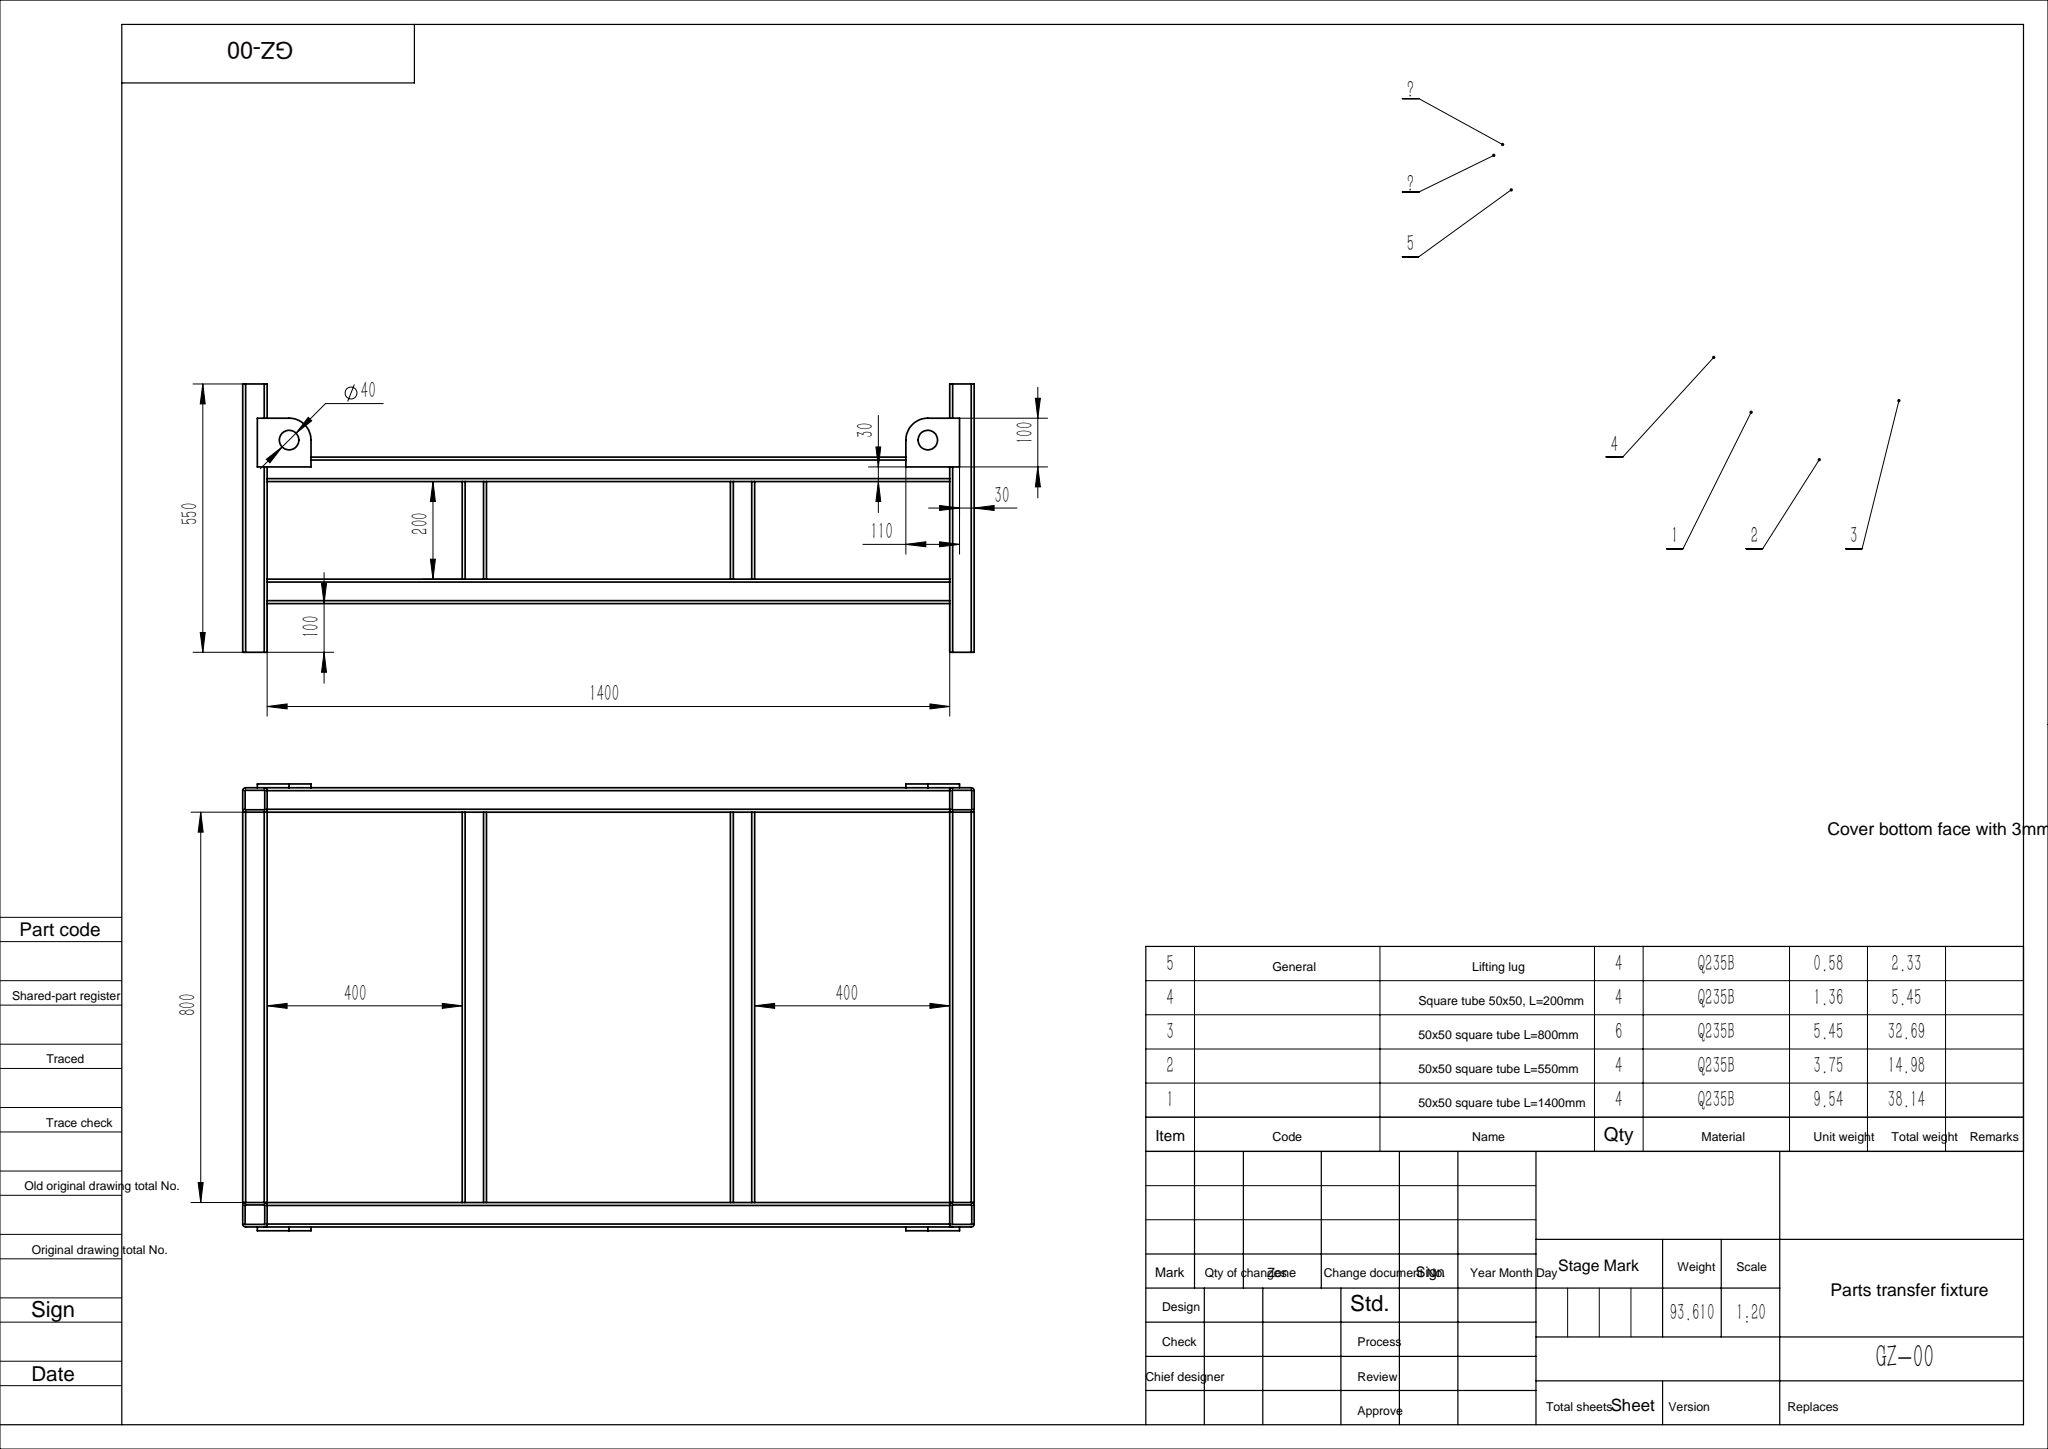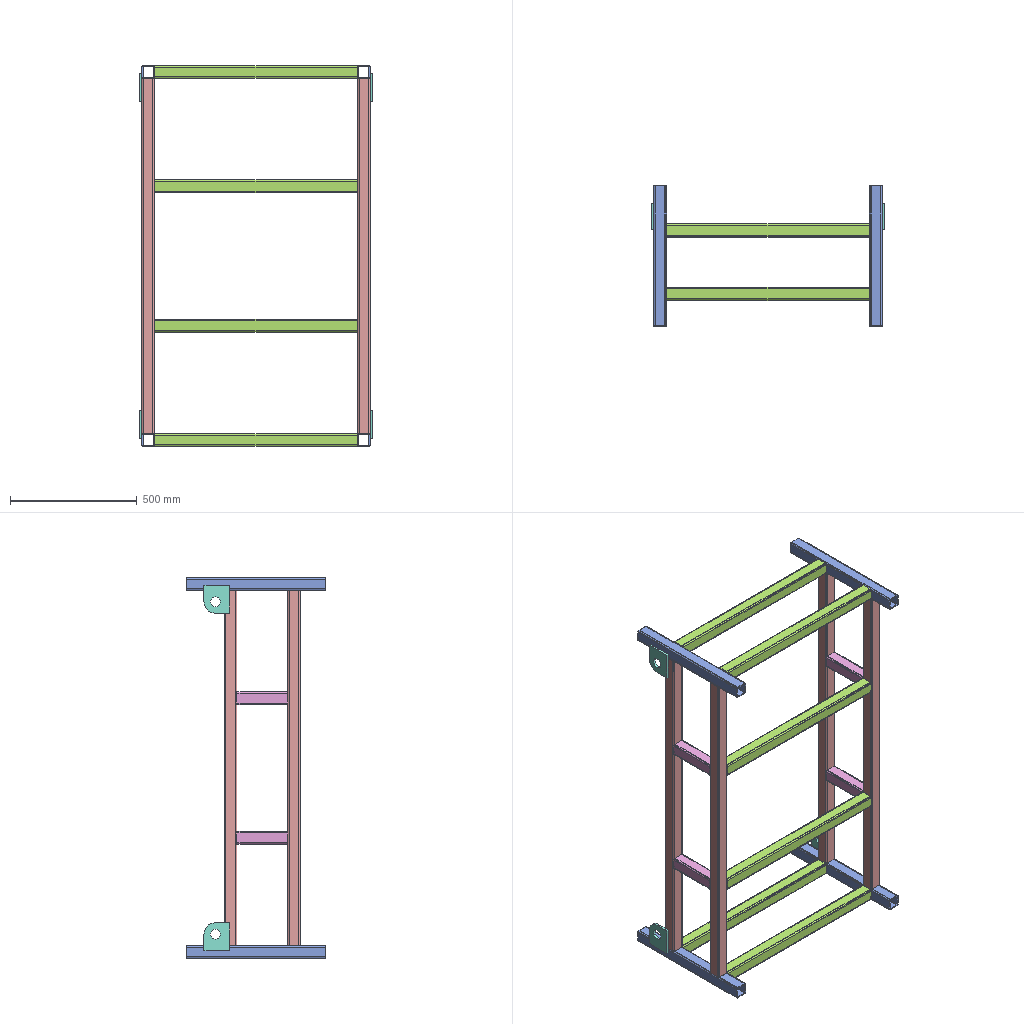Assembly | SolidWorks | 5 different items | 22 placed | box 916 x 550 x 1500 mm
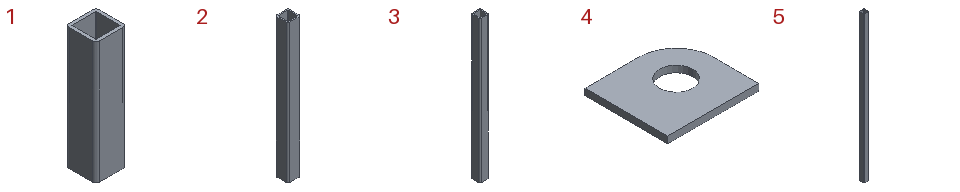Parts list (item | quantity | size | volume | features):
1 | x4 | 50 x 50 x 200 mm | 173991 mm3 | features Extrusion 1
2 | x4 | 50 x 50 x 550 mm | 478476 mm3 | features Extrusion 1
3 | x6 | 50 x 50 x 800 mm | 695965 mm3 | features Extrusion 1
4 | x4 | 110 x 100 x 8 mm | 74470 mm3 | features Extrusion 1
5 | x4 | 50 x 50 x 1400 mm | 1217938 mm3 | features Extrusion 1
Mates (type | each side: item.copy, entity, surface, feature):
Coincident | 5.1 face plane Boss-Extrude1 | 2.1 face plane Boss-Extrude1 | 2 times
DistanceDim | 5.1 face plane Boss-Extrude1 | 2.1 face plane Boss-Extrude1
Coincident | 5.1 face plane Boss-Extrude1 | 3.1 face plane Boss-Extrude1
Coincident | 2.1 face plane Boss-Extrude1 | 3.1 face plane Boss-Extrude1 | 2 times
Coincident | 3.1 face plane Boss-Extrude1 | 2.2 face plane Boss-Extrude1 | 2 times
Coincident | 2.1 face plane Boss-Extrude1 | 2.2 face plane Boss-Extrude1
Coincident | 2.1 face plane Boss-Extrude1 | 2.3 face plane Boss-Extrude1
Coincident | 2.1 face plane Boss-Extrude1 | 2.4 face plane Boss-Extrude1
Coincident | 3.1 face plane Boss-Extrude1 | 5.2 face plane Boss-Extrude1
Coincident | 5.2 face plane Boss-Extrude1 | 2.2 face plane Boss-Extrude1 | 2 times
Coincident | 5.2 face plane Boss-Extrude1 | 2.3 face plane Boss-Extrude1 | 2 times
Coincident | 5.1 face plane Boss-Extrude1 | 2.4 face plane Boss-Extrude1 | 2 times
Coincident | 5.1 face plane Boss-Extrude1 | 3.2 face plane Boss-Extrude1
Coincident | 2.3 face plane Boss-Extrude1 | 3.2 face plane Boss-Extrude1
Coincident | 2.4 face plane Boss-Extrude1 | 3.2 face plane Boss-Extrude1
Coincident | 5.2 face plane Boss-Extrude1 | 3.3 face plane Boss-Extrude1 | 2 times
Coincident | 2.1 face plane Boss-Extrude1 | 5.3 face plane Boss-Extrude1 | 2 times
DistanceDim | 5.3 face plane Boss-Extrude1 | 2.1 face plane Boss-Extrude1
Coincident | 2.2 face plane Boss-Extrude1 | 5.4 face plane Boss-Extrude1 | 2 times
Coincident | 5.3 face plane Boss-Extrude1 | 5.4 face plane Boss-Extrude1
Coincident | 5.3 face plane Boss-Extrude1 | 3.4 face plane Boss-Extrude1
Coincident | 2.1 face plane Boss-Extrude1 | 3.4 face plane Boss-Extrude1
Coincident | 2.2 face plane Boss-Extrude1 | 3.4 face plane Boss-Extrude1
Coincident | 5.3 face plane Boss-Extrude1 | 3.5 face plane Boss-Extrude1
Coincident | 2.3 face plane Boss-Extrude1 | 3.5 face plane Boss-Extrude1 | 2 times
Coincident | 5.2 face plane Boss-Extrude1 | 1.1 face plane Boss-Extrude1 | 2 times
Coincident | 5.2 face plane Boss-Extrude1 | 1.2 face plane Boss-Extrude1
Coincident | 5.4 face plane Boss-Extrude1 | 1.2 face plane Boss-Extrude1
Coincident | 5.3 face plane Boss-Extrude1 | 1.3 face plane Boss-Extrude1 | 2 times
Coincident | 5.3 face plane Boss-Extrude1 | 1.4 face plane Boss-Extrude1
Coincident | 5.1 face plane Boss-Extrude1 | 1.4 face plane Boss-Extrude1
Coincident | 1.1 face plane Boss-Extrude1 | 1.4 face plane Boss-Extrude1
Coincident | 1.2 face plane Boss-Extrude1 | 1.3 face plane Boss-Extrude1
DistanceDim | 1.3 face plane Boss-Extrude1 | 2.1 face plane Boss-Extrude1
DistanceDim | 1.4 face plane Boss-Extrude1 | 2.4 face plane Boss-Extrude1
Coincident | 3.3 face plane Boss-Extrude1 | 1.2 face plane Boss-Extrude1
Coincident | 5.1 face plane Boss-Extrude1 | 3.6 face plane Boss-Extrude1 | 2 times
Coincident | 1.4 face plane Boss-Extrude1 | 3.6 face plane Boss-Extrude1
Coincident | 2.2 face plane Boss-Extrude1 | 4.1 face plane Boss-Extrude1
DistanceDim | 4.1 face plane Boss-Extrude1 | 2.2 face plane Boss-Extrude1
DistanceDim | 4.1 face plane Boss-Extrude1 | 5.4 face plane Boss-Extrude1
Coincident | 2.3 face plane Boss-Extrude1 | 4.2 face plane Boss-Extrude1
DistanceDim | 4.2 face plane Boss-Extrude1 | 2.3 face plane Boss-Extrude1
DistanceDim | 4.2 face plane Boss-Extrude1 | 5.4 face plane Boss-Extrude1
Coincident | 2.4 face plane Boss-Extrude1 | 4.3 face plane Boss-Extrude1
DistanceDim | 4.3 face plane Boss-Extrude1 | 2.4 face plane Boss-Extrude1
DistanceDim | 4.3 face plane Boss-Extrude1 | 5.3 face plane Boss-Extrude1
Coincident | 2.1 face plane Boss-Extrude1 | 4.4 face plane Boss-Extrude1
DistanceDim | 4.4 face plane Boss-Extrude1 | 2.1 face plane Boss-Extrude1
DistanceDim | 4.4 face plane Boss-Extrude1 | 5.3 face plane Boss-Extrude1